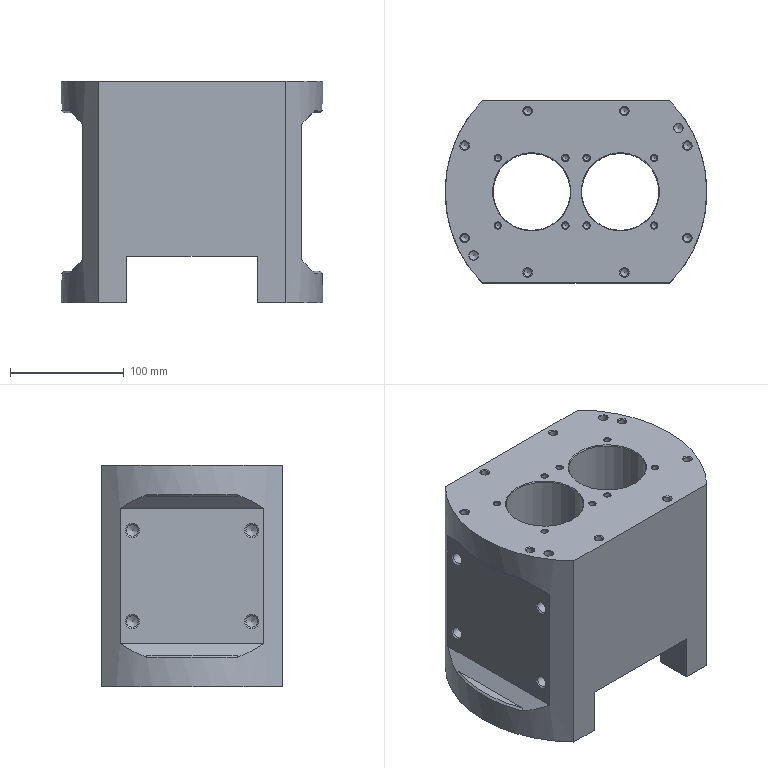NC program | NX | posted with a generic post | part box 230 x 160 x 195 mm
Lines 1 to 673 of 6546:
N10 G17 G21 G94 G90
(FLOOR_WALL_COPY_1_COPY , TOOL : D50)
N12 T02 M6
N14 G54
N16 G17 G0 G90 X34.597 Y36.969 B0. C0. S1200 M3
N18 G43 Z30. H2
N20 Z2.65
N22 G94 G1 Z-0.35 F1000.
N24 Y33.969
N26 Y-33.969 F2000.
N28 X-0.001
N30 Y33.969
N32 X-34.6
N34 Y-33.969
N36 Y-36.969
N38 Z2.65
N40 G0 Z30.
N42 X34.597 Y40.672
N44 Z2.3
N46 G1 Z-0.7 F1000.
N48 Y37.672
N50 Y-37.672 F2000.
N52 X-0.001
N54 Y37.672
N56 X-34.6
N58 Y-37.672
N60 Y-40.672
N62 Z2.3
N64 G0 Z30.
N66 X34.597 Y43.507
N68 Z1.95
N70 G1 Z-1.05 F1000.
N72 Y40.507
N74 Y-40.507 F2000.
N76 X-0.001
N78 Y40.507
N80 X-34.6
N82 Y-40.507
N84 Y-43.507
N86 Z1.95
N88 G0 Z30.
N90 X34.597 Y45.891
N92 Z1.6
N94 G1 Z-1.4 F1000.
N96 Y42.891
N98 Y-42.891 F2000.
N100 X-0.001
N102 Y42.891
N104 X-34.6
N106 Y-42.891
N108 Y-45.891
N110 Z1.6
N112 G0 Z30.
N114 X34.597 Y47.987
N116 Z1.25
N118 G1 Z-1.75 F1000.
N120 Y44.987
N122 Y-44.987 F2000.
N124 X-0.001
N126 Y44.987
N128 X-34.6
N130 Y-44.987
N132 Y-47.987
N134 Z1.25
N136 G0 Z30.
N138 X34.597 Y49.878
N140 Z0.9
N142 G1 Z-2.1 F1000.
N144 Y46.878
N146 Y-46.878 F2000.
N148 X-0.001
N150 Y46.878
N152 X-34.6
N154 Y-46.878
N156 Y-49.878
N158 Z0.9
N160 G0 Z30.
N162 X34.597 Y51.613
N164 Z0.55
N166 G1 Z-2.45 F1000.
N168 Y48.613
N170 Y-48.613 F2000.
N172 X-0.001
N174 Y48.613
N176 X-34.6
N178 Y-48.613
N180 Y-51.613
N182 Z0.55
N184 G0 Z30.
N186 X34.597 Y53.223
N188 Z0.2
N190 G1 Z-2.8 F1000.
N192 Y50.223
N194 Y-50.223 F2000.
N196 X-0.001
N198 Y50.223
N200 X-34.6
N202 Y-50.223
N204 Y-53.223
N206 Z0.2
N208 G0 Z30.
N210 X34.597 Y54.733
N212 Z-0.15
N214 G1 Z-3.15 F1000.
N216 Y51.733
N218 Y-51.733 F2000.
N220 X-0.001
N222 Y51.733
N224 X-34.6
N226 Y-51.733
N228 Y-54.733
N230 Z-0.15
N232 G0 Z30.
N234 X34.597 Y56.157
N236 Z-0.5
N238 G1 Z-3.5 F1000.
N240 Y53.157
N242 Y-53.157 F2000.
N244 X-0.001
N246 Y53.157
N248 X-34.6
N250 Y-53.157
N252 Y-56.157
N254 Z-0.5
N256 G0 Z30.
N258 X34.597 Y57.508
N260 Z-0.85
N262 G1 Z-3.85 F1000.
N264 Y54.508
N266 Y-54.508 F2000.
N268 X-0.001
N270 Y54.508
N272 X-34.6
N274 Y-54.508
N276 Y-57.508
N278 Z-0.85
N280 G0 Z30.
N282 X34.597 Y58.796
N284 Z-1.2
N286 G1 Z-4.2 F1000.
N288 Y55.796
N290 Y-55.796 F2000.
N292 X-0.001
N294 Y55.796
N296 X-34.6
N298 Y-55.796
N300 Y-58.796
N302 Z-1.2
N304 G0 Z30.
N306 X34.597 Y60.029
N308 Z-1.55
N310 G1 Z-4.55 F1000.
N312 Y57.029
N314 Y-57.029 F2000.
N316 X-0.001
N318 Y57.029
N320 X-34.6
N322 Y-57.029
N324 Y-60.029
N326 Z-1.55
N328 G0 Z30.
N330 X34.597 Y61.212
N332 Z-1.9
N334 G1 Z-4.9 F1000.
N336 Y58.212
N338 Y-58.212 F2000.
N340 X-0.001
N342 Y58.212
N344 X-34.6
N346 Y-58.212
N348 Y-61.212
N350 Z-1.9
N352 G0 Z30.
N354 X34.597 Y62.351
N356 Z-2.25
N358 G1 Z-5.25 F1000.
N360 Y59.351
N362 Y-59.351 F2000.
N364 X-0.001
N366 Y59.351
N368 X-34.6
N370 Y-59.351
N372 Y-62.351
N374 Z-2.25
N376 G0 Z30.
N378 X34.597 Y63.45
N380 Z-2.6
N382 G1 Z-5.6 F1000.
N384 Y60.45
N386 Y-60.45 F2000.
N388 X-0.001
N390 Y60.45
N392 X-34.6
N394 Y-60.45
N396 Y-63.45
N398 Z-2.6
N400 G0 Z30.
N402 X34.597 Y64.512
N404 Z-2.95
N406 G1 Z-5.95 F1000.
N408 Y61.512
N410 Y-61.512 F2000.
N412 X-0.001
N414 Y61.512
N416 X-34.6
N418 Y-61.512
N420 Y-64.512
N422 Z-2.95
N424 G0 Z30.
N426 X34.597 Y65.541
N428 Z-3.3
N430 G1 Z-6.3 F1000.
N432 Y62.541
N434 Y-62.541 F2000.
N436 X-0.001
N438 Y62.541
N440 X-34.6
N442 Y-62.541
N444 Y-65.541
N446 Z-3.3
N448 G0 Z30.
N450 X34.597 Y66.54
N452 Z-3.65
N454 G1 Z-6.65 F1000.
N456 Y63.54
N458 Y-63.54 F2000.
N460 X-0.001
N462 Y63.54
N464 X-34.6
N466 Y-63.54
N468 Y-66.54
N470 Z-3.65
N472 G0 Z30.
N474 X34.597 Y67.51
N476 Z-4.
N478 G1 Z-7. F1000.
N480 Y64.51
N482 Y-64.51 F2000.
N484 X-0.001
N486 Y64.51
N488 X-34.6
N490 Y-64.51
N492 Y-67.51
N494 Z-4.
N496 G0 Z30.
N498 X34.597 Y68.454
N500 Z-4.35
N502 G1 Z-7.35 F1000.
N504 Y65.454
N506 Y-65.454 F2000.
N508 X-0.001
N510 Y65.454
N512 X-34.6
N514 Y-65.454
N516 Y-68.454
N518 Z-4.35
N520 G0 Z30.
N522 X34.597 Y69.373
N524 Z-4.7
N526 G1 Z-7.7 F1000.
N528 Y66.373
N530 Y-66.373 F2000.
N532 X-0.001
N534 Y66.373
N536 X-34.6
N538 Y-66.373
N540 Y-69.373
N542 Z-4.7
N544 G0 Z30.
N546 X34.597 Y70.27
N548 Z-5.05
N550 G1 Z-8.05 F1000.
N552 Y67.27
N554 Y-67.27 F2000.
N556 X-0.001
N558 Y67.27
N560 X-34.6
N562 Y-67.27
N564 Y-70.27
N566 Z-5.05
N568 G0 Z30.
N570 X34.597 Y71.145
N572 Z-5.4
N574 G1 Z-8.4 F1000.
N576 Y68.145
N578 Y-68.145 F2000.
N580 X-0.001
N582 Y68.145
N584 X-34.6
N586 Y-68.145
N588 Y-71.145
N590 Z-5.4
N592 G0 Z30.
N594 X34.597 Y72.
N596 Z-5.75
N598 G1 Z-8.75 F1000.
N600 Y69.
N602 Y-69. F2000.
N604 X-0.001
N606 Y69.
N608 X-34.6
N610 Y-69.
N612 Y-72.
N614 Z-5.75
N616 G0 Z30.
N618 X34.597 Y72.836
N620 Z-6.1
N622 G1 Z-9.1 F1000.
N624 Y69.836
N626 Y-69.836 F2000.
N628 X-0.001
N630 Y69.836
N632 X-34.6
N634 Y-69.836
N636 Y-72.836
N638 Z-6.1
N640 G0 Z30.
N642 X34.597 Y73.653
N644 Z-6.45
N646 G1 Z-9.45 F1000.
N648 Y70.653
N650 Y-70.653 F2000.
N652 X-0.001
N654 Y70.653
N656 X-34.6
N658 Y-70.653
N660 Y-73.653
N662 Z-6.45
N664 G0 Z30.
N666 X34.597 Y74.454
N668 Z-6.8
N670 G1 Z-9.8 F1000.
N672 Y71.454
N674 Y-71.454 F2000.
N676 X-0.001
N678 Y71.454
N680 X-34.6
N682 Y-71.454
N684 Y-74.454
N686 Z-6.8
N688 G0 Z30.
N690 X34.597 Y75.239
N692 Z-7.15
N694 G1 Z-10.15 F1000.
N696 Y72.239
N698 Y-72.239 F2000.
N700 X-0.001
N702 Y72.239
N704 X-34.6
N706 Y-72.239
N708 Y-75.239
N710 Z-7.15
N712 G0 Z30.
N714 X34.597 Y76.008
N716 Z-7.5
N718 G1 Z-10.5 F1000.
N720 Y73.008
N722 Y-73.008 F2000.
N724 X-0.001
N726 Y73.008
N728 X-34.6
N730 Y-73.008
N732 Y-76.008
N734 Z-7.5
N736 G0 Z30.
N738 X34.597 Y76.763
N740 Z-7.85
N742 G1 Z-10.85 F1000.
N744 Y73.763
N746 Y-73.763 F2000.
N748 X-0.001
N750 Y73.763
N752 X-34.6
N754 Y-73.763
N756 Y-76.763
N758 Z-7.85
N760 G0 Z30.
N762 X34.597 Y77.503
N764 Z-8.2
N766 G1 Z-11.2 F1000.
N768 Y74.503
N770 Y-74.503 F2000.
N772 X-0.001
N774 Y74.503
N776 X-34.6
N778 Y-74.503
N780 Y-77.503
N782 Z-8.2
N784 G0 Z30.
N786 X34.597 Y78.231
N788 Z-8.55
N790 G1 Z-11.55 F1000.
N792 Y75.231
N794 Y-75.231 F2000.
N796 X-0.001
N798 Y75.231
N800 X-34.6
N802 Y-75.231
N804 Y-78.231
N806 Z-8.55
N808 G0 Z30.
N810 X34.597 Y78.945
N812 Z-8.9
N814 G1 Z-11.9 F1000.
N816 Y75.945
N818 Y-75.945 F2000.
N820 X-0.001
N822 Y75.945
N824 X-34.6
N826 Y-75.945
N828 Y-78.945
N830 Z-8.9
N832 G0 Z30.
N834 X34.597 Y79.647
N836 Z-9.25
N838 G1 Z-12.25 F1000.
N840 Y76.647
N842 Y-76.647 F2000.
N844 X-0.001
N846 Y76.647
N848 X-34.6
N850 Y-76.647
N852 Y-79.647
N854 Z-9.25
N856 G0 Z30.
N858 X34.597 Y80.338
N860 Z-9.6
N862 G1 Z-12.6 F1000.
N864 Y77.338
N866 Y-77.338 F2000.
N868 X-0.001
N870 Y77.338
N872 X-34.6
N874 Y-77.338
N876 Y-80.338
N878 Z-9.6
N880 G0 Z30.
N882 X34.597 Y81.017
N884 Z-9.95
N886 G1 Z-12.95 F1000.
N888 Y78.017
N890 Y-78.017 F2000.
N892 X-0.001
N894 Y78.017
N896 X-34.6
N898 Y-78.017
N900 Y-81.017
N902 Z-9.95
N904 G0 Z30.
N906 X34.597 Y81.685
N908 Z-10.3
N910 G1 Z-13.3 F1000.
N912 Y78.685
N914 Y-78.685 F2000.
N916 X-0.001
N918 Y78.685
N920 X-34.6
N922 Y-78.685
N924 Y-81.685
N926 Z-10.3
N928 G0 Z30.
N930 X34.597 Y82.343
N932 Z-10.65
N934 G1 Z-13.65 F1000.
N936 Y79.343
N938 Y-79.343 F2000.
N940 X-0.001
N942 Y79.343
N944 X-34.6
N946 Y-79.343
N948 Y-82.343
N950 Z-10.65
N952 G0 Z30.
N954 X34.597 Y82.991
N956 Z-11.
N958 G1 Z-14. F1000.
N960 Y79.991
N962 Y-79.991 F2000.
N964 X-0.001
N966 Y79.991
N968 X-34.6
N970 Y-79.991
N972 Y-82.991
N974 Z-11.
N976 G0 Z30.
N978 X34.597 Y83.629
N980 Z-11.35
N982 G1 Z-14.35 F1000.
N984 Y80.629
N986 Y-80.629 F2000.
N988 X-0.001
N990 Y80.629
N992 X-34.6
N994 Y-80.629
N996 Y-83.629
N998 Z-11.35
N1000 G0 Z30.
N1002 X34.597 Y84.258
N1004 Z-11.7
N1006 G1 Z-14.7 F1000.
N1008 Y81.258
N1010 Y-81.258 F2000.
N1012 X-0.001
N1014 Y81.258
N1016 X-34.6
N1018 Y-81.258
N1020 Y-84.258
N1022 Z-11.7
N1024 G0 Z30.
N1026 X34.597 Y84.877
N1028 Z-12.05
N1030 G1 Z-15.05 F1000.
N1032 Y81.877
N1034 Y-81.877 F2000.
N1036 X-0.001
N1038 Y81.877
N1040 X-34.6
N1042 Y-81.877
N1044 Y-84.877
N1046 Z-12.05
N1048 G0 Z30.
N1050 X34.597 Y85.488
N1052 Z-12.4
N1054 G1 Z-15.4 F1000.
N1056 Y82.488
N1058 Y-82.488 F2000.
N1060 X-0.001
N1062 Y82.488
N1064 X-34.6
N1066 Y-82.488
N1068 Y-85.488
N1070 Z-12.4
N1072 G0 Z30.
N1074 X34.597 Y86.09
N1076 Z-12.75
N1078 G1 Z-15.75 F1000.
N1080 Y83.09
N1082 Y-83.09 F2000.
N1084 X-0.001
N1086 Y83.09
N1088 X-34.6
N1090 Y-83.09
N1092 Y-86.09
N1094 Z-12.75
N1096 G0 Z30.
N1098 X34.597 Y86.684
N1100 Z-13.1
N1102 G1 Z-16.1 F1000.
N1104 Y83.684
N1106 Y-83.684 F2000.
N1108 X-0.001
N1110 Y83.684
N1112 X-34.6
N1114 Y-83.684
N1116 Y-86.684
N1118 Z-13.1
N1120 G0 Z30.
N1122 X34.597 Y87.27
N1124 Z-13.45
N1126 G1 Z-16.45 F1000.
N1128 Y84.27
N1130 Y-84.27 F2000.
N1132 X-0.001
N1134 Y84.27
N1136 X-34.6
N1138 Y-84.27
N1140 Y-87.27
N1142 Z-13.45
N1144 G0 Z30.
N1146 X34.597 Y87.848
N1148 Z-13.8
N1150 G1 Z-16.8 F1000.
N1152 Y84.848
N1154 Y-84.848 F2000.
N1156 X-0.001
N1158 Y84.848
N1160 X-34.6
N1162 Y-84.848
N1164 Y-87.848
N1166 Z-13.8
N1168 G0 Z30.
N1170 X34.597 Y88.418
N1172 Z-14.15
N1174 G1 Z-17.15 F1000.
N1176 Y85.418
N1178 Y-85.418 F2000.
N1180 X-0.001
N1182 Y85.418
N1184 X-34.6
N1186 Y-85.418
N1188 Y-88.418
N1190 Z-14.15
N1192 G0 Z30.
N1194 X34.597 Y88.982
N1196 Z-14.5
N1198 G1 Z-17.5 F1000.
N1200 Y85.982
N1202 Y-85.982 F2000.
N1204 X-0.001
N1206 Y85.982
N1208 X-34.6
N1210 Y-85.982
N1212 Y-88.982
N1214 Z-14.5
N1216 G0 Z30.
N1218 X34.597 Y89.538
N1220 Z-14.85
N1222 G1 Z-17.85 F1000.
N1224 Y86.538
N1226 Y-86.538 F2000.
N1228 X-0.001
N1230 Y86.538
N1232 X-34.6
N1234 Y-86.538
N1236 Y-89.538
N1238 Z-14.85
N1240 G0 Z30.
N1242 X34.597 Y90.087
N1244 Z-15.2
N1246 G1 Z-18.2 F1000.
N1248 Y87.087
N1250 Y-87.087 F2000.
N1252 X-0.001
N1254 Y87.087
N1256 X-34.6
N1258 Y-87.087
N1260 Y-90.087
N1262 Z-15.2
N1264 G0 Z30.
N1266 X34.597 Y90.629
N1268 Z-15.55
N1270 G1 Z-18.55 F1000.
N1272 Y87.629
N1274 Y-87.629 F2000.
N1276 X-0.001
N1278 Y87.629
N1280 X-34.6
N1282 Y-87.629
N1284 Y-90.629
N1286 Z-15.55
N1288 G0 Z30.
N1290 X34.597 Y91.165
N1292 Z-15.9
N1294 G1 Z-18.9 F1000.
N1296 Y88.165
N1298 Y-88.165 F2000.
N1300 X-0.001
N1302 Y88.165
N1304 X-34.6
N1306 Y-88.165
N1308 Y-91.165
N1310 Z-15.9
N1312 G0 Z30.
(FLOOR_WALL_COPY_COPY_COPY , TOOL : D50)
N1314 X34.497 Y91.317 S2500
N1316 Z-16.
N1318 G1 Z-19. F1000.
N1320 Y88.317
N1322 Y-88.317
N1324 X-0.001
N1326 Y88.317
N1328 X-34.5
N1330 Y-88.317
N1332 Y-91.317
N1334 Z-16.
N1336 G0 Z30.
N1338 M5